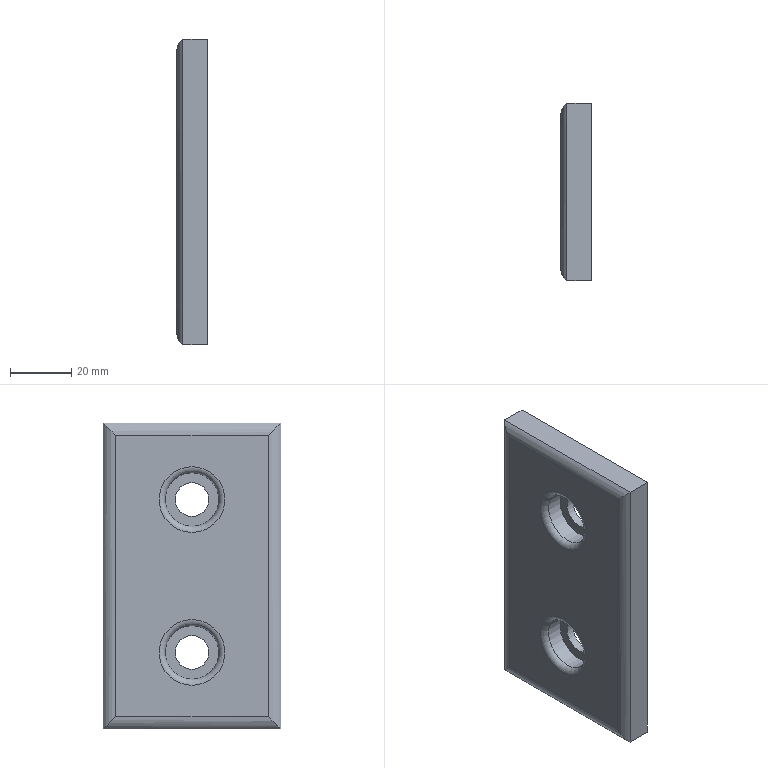Part | STEP file | lll_id5046_x_t | 1 solid | 18 faces | box 10 x 58 x 100 mm | volume 53133 mm3 | plane 8 | cylinder 8 | torus 2 | commonest cylinder face diameters 10 x4 11 x2 17.5 x2
STEP:
#1=CARTESIAN_POINT('',(2835.,334.047,9.));
#2=VERTEX_POINT('',#1);
#3=CARTESIAN_POINT('',(2835.,284.047,9.));
#4=VERTEX_POINT('',#3);
#5=CARTESIAN_POINT('',(2835.,323.047,9.));
#6=DIRECTION('',(0.,-1.,0.));
#7=VECTOR('',#6,1.);
#8=LINE('',#5,#7);
#9=EDGE_CURVE('',#2,#4,#8,.T.);
#10=ORIENTED_EDGE('',*,*,#9,.T.);
#11=CARTESIAN_POINT('',(2835.,284.047,101.));
#12=VERTEX_POINT('',#11);
#13=CARTESIAN_POINT('',(2835.,284.047,105.));
#14=DIRECTION('',(0.,0.,-1.));
#15=VECTOR('',#14,1.);
#16=LINE('',#13,#15);
#17=EDGE_CURVE('',#12,#4,#16,.T.);
#18=ORIENTED_EDGE('',*,*,#17,.F.);
#19=CARTESIAN_POINT('',(2835.,334.047,101.));
#20=VERTEX_POINT('',#19);
#21=CARTESIAN_POINT('',(2835.,323.047,101.));
#22=DIRECTION('',(0.,-1.,0.));
#23=VECTOR('',#22,1.);
#24=LINE('',#21,#23);
#25=EDGE_CURVE('',#20,#12,#24,.T.);
#26=ORIENTED_EDGE('',*,*,#25,.F.);
#27=CARTESIAN_POINT('',(2835.,334.047,105.));
#28=DIRECTION('',(0.,0.,-1.));
#29=VECTOR('',#28,1.);
#30=LINE('',#27,#29);
#31=EDGE_CURVE('',#20,#2,#30,.T.);
#32=ORIENTED_EDGE('',*,*,#31,.T.);
#33=EDGE_LOOP('',(#10,#18,#26,#32));
#34=FACE_BOUND('',#33,.T.);
#35=CARTESIAN_POINT('',(2835.,309.047,69.25));
#36=VERTEX_POINT('',#35);
#37=CARTESIAN_POINT('',(2835.,309.047,80.));
#38=DIRECTION('',(1.,0.,0.));
#39=DIRECTION('',(0.,0.,-1.));
#40=AXIS2_PLACEMENT_3D('',#37,#38,#39);
#41=CIRCLE('',#40,10.75);
#42=EDGE_CURVE('',#36,#36,#41,.T.);
#43=ORIENTED_EDGE('',*,*,#42,.T.);
#44=EDGE_LOOP('',(#43));
#45=FACE_BOUND('',#44,.T.);
#46=CARTESIAN_POINT('',(2835.,309.047,19.25));
#47=VERTEX_POINT('',#46);
#48=CARTESIAN_POINT('',(2835.,309.047,30.));
#49=DIRECTION('',(1.,0.,0.));
#50=DIRECTION('',(0.,0.,-1.));
#51=AXIS2_PLACEMENT_3D('',#48,#49,#50);
#52=CIRCLE('',#51,10.75);
#53=EDGE_CURVE('',#47,#47,#52,.T.);
#54=ORIENTED_EDGE('',*,*,#53,.T.);
#55=EDGE_LOOP('',(#54));
#56=FACE_BOUND('',#55,.T.);
#57=CARTESIAN_POINT('',(2835.,295.047,-20.));
#58=DIRECTION('',(-1.,0.,0.));
#59=DIRECTION('',(0.,0.,-1.));
#60=AXIS2_PLACEMENT_3D('',#57,#58,#59);
#61=PLANE('',#60);
#62=ADVANCED_FACE('',(#34,#45,#56),#61,.T.);
#63=CARTESIAN_POINT('',(2845.,309.047,24.5));
#64=VERTEX_POINT('',#63);
#65=CARTESIAN_POINT('',(2845.,309.047,30.));
#66=DIRECTION('',(1.,0.,0.));
#67=DIRECTION('',(0.,0.,-1.));
#68=AXIS2_PLACEMENT_3D('',#65,#66,#67);
#69=CIRCLE('',#68,5.5);
#70=EDGE_CURVE('',#64,#64,#69,.T.);
#71=ORIENTED_EDGE('',*,*,#70,.T.);
#72=EDGE_LOOP('',(#71));
#73=FACE_BOUND('',#72,.T.);
#74=CARTESIAN_POINT('',(2842.3,309.047,24.5));
#75=VERTEX_POINT('',#74);
#76=CARTESIAN_POINT('',(2842.3,309.047,30.));
#77=DIRECTION('',(1.,0.,0.));
#78=DIRECTION('',(0.,0.,-1.));
#79=AXIS2_PLACEMENT_3D('',#76,#77,#78);
#80=CIRCLE('',#79,5.5);
#81=EDGE_CURVE('',#75,#75,#80,.T.);
#82=ORIENTED_EDGE('',*,*,#81,.F.);
#83=EDGE_LOOP('',(#82));
#84=FACE_BOUND('',#83,.T.);
#85=CARTESIAN_POINT('',(2934.,309.047,30.));
#86=DIRECTION('',(-1.,0.,0.));
#87=DIRECTION('',(0.,0.,-1.));
#88=AXIS2_PLACEMENT_3D('',#85,#86,#87);
#89=CYLINDRICAL_SURFACE('',#88,5.5);
#90=ADVANCED_FACE('',(#73,#84),#89,.F.);
#91=CARTESIAN_POINT('',(2845.,338.047,5.));
#92=VERTEX_POINT('',#91);
#93=CARTESIAN_POINT('',(2845.,280.047,5.));
#94=VERTEX_POINT('',#93);
#95=CARTESIAN_POINT('',(2845.,323.047,5.));
#96=DIRECTION('',(0.,-1.,0.));
#97=VECTOR('',#96,1.);
#98=LINE('',#95,#97);
#99=EDGE_CURVE('',#92,#94,#98,.T.);
#100=ORIENTED_EDGE('',*,*,#99,.F.);
#101=CARTESIAN_POINT('',(2845.,338.047,105.));
#102=VERTEX_POINT('',#101);
#103=CARTESIAN_POINT('',(2845.,338.047,105.));
#104=DIRECTION('',(0.,0.,-1.));
#105=VECTOR('',#104,1.);
#106=LINE('',#103,#105);
#107=EDGE_CURVE('',#102,#92,#106,.T.);
#108=ORIENTED_EDGE('',*,*,#107,.F.);
#109=CARTESIAN_POINT('',(2845.,280.047,105.));
#110=VERTEX_POINT('',#109);
#111=CARTESIAN_POINT('',(2845.,295.047,105.));
#112=DIRECTION('',(0.,1.,0.));
#113=VECTOR('',#112,1.);
#114=LINE('',#111,#113);
#115=EDGE_CURVE('',#110,#102,#114,.T.);
#116=ORIENTED_EDGE('',*,*,#115,.F.);
#117=CARTESIAN_POINT('',(2845.,280.047,-20.));
#118=DIRECTION('',(0.,0.,1.));
#119=VECTOR('',#118,1.);
#120=LINE('',#117,#119);
#121=EDGE_CURVE('',#94,#110,#120,.T.);
#122=ORIENTED_EDGE('',*,*,#121,.F.);
#123=EDGE_LOOP('',(#100,#108,#116,#122));
#124=FACE_BOUND('',#123,.T.);
#125=ORIENTED_EDGE('',*,*,#70,.F.);
#126=EDGE_LOOP('',(#125));
#127=FACE_BOUND('',#126,.T.);
#128=CARTESIAN_POINT('',(2845.,309.047,74.5));
#129=VERTEX_POINT('',#128);
#130=CARTESIAN_POINT('',(2845.,309.047,80.));
#131=DIRECTION('',(-1.,0.,0.));
#132=DIRECTION('',(0.,0.,-1.));
#133=AXIS2_PLACEMENT_3D('',#130,#131,#132);
#134=CIRCLE('',#133,5.5);
#135=EDGE_CURVE('',#129,#129,#134,.T.);
#136=ORIENTED_EDGE('',*,*,#135,.T.);
#137=EDGE_LOOP('',(#136));
#138=FACE_BOUND('',#137,.T.);
#139=CARTESIAN_POINT('',(2845.,295.047,-20.));
#140=DIRECTION('',(-1.,0.,0.));
#141=DIRECTION('',(0.,0.,-1.));
#142=AXIS2_PLACEMENT_3D('',#139,#140,#141);
#143=PLANE('',#142);
#144=ADVANCED_FACE('',(#124,#127,#138),#143,.F.);
#145=CARTESIAN_POINT('',(2837.,280.047,105.));
#146=VERTEX_POINT('',#145);
#147=CARTESIAN_POINT('',(2835.,280.047,105.));
#148=DIRECTION('',(1.,0.,0.));
#149=VECTOR('',#148,1.);
#150=LINE('',#147,#149);
#151=EDGE_CURVE('',#146,#110,#150,.T.);
#152=ORIENTED_EDGE('',*,*,#151,.F.);
#153=CARTESIAN_POINT('',(2837.,280.047,5.));
#154=VERTEX_POINT('',#153);
#155=CARTESIAN_POINT('',(2837.,280.047,105.));
#156=DIRECTION('',(0.,0.,-1.));
#157=VECTOR('',#156,1.);
#158=LINE('',#155,#157);
#159=EDGE_CURVE('',#146,#154,#158,.T.);
#160=ORIENTED_EDGE('',*,*,#159,.T.);
#161=CARTESIAN_POINT('',(2835.,280.047,5.));
#162=DIRECTION('',(1.,0.,0.));
#163=VECTOR('',#162,1.);
#164=LINE('',#161,#163);
#165=EDGE_CURVE('',#154,#94,#164,.T.);
#166=ORIENTED_EDGE('',*,*,#165,.T.);
#167=ORIENTED_EDGE('',*,*,#121,.T.);
#168=EDGE_LOOP('',(#152,#160,#166,#167));
#169=FACE_OUTER_BOUND('',#168,.T.);
#170=CARTESIAN_POINT('',(2835.,280.047,-20.));
#171=DIRECTION('',(0.,1.,0.));
#172=DIRECTION('',(1.,0.,0.));
#173=AXIS2_PLACEMENT_3D('',#170,#171,#172);
#174=PLANE('',#173);
#175=ADVANCED_FACE('',(#169),#174,.F.);
#176=CARTESIAN_POINT('',(2837.,338.047,105.));
#177=VERTEX_POINT('',#176);
#178=CARTESIAN_POINT('',(2837.,323.047,105.));
#179=DIRECTION('',(0.,-1.,0.));
#180=VECTOR('',#179,1.);
#181=LINE('',#178,#180);
#182=EDGE_CURVE('',#177,#146,#181,.T.);
#183=ORIENTED_EDGE('',*,*,#182,.T.);
#184=ORIENTED_EDGE('',*,*,#151,.T.);
#185=ORIENTED_EDGE('',*,*,#115,.T.);
#186=CARTESIAN_POINT('',(2835.,338.047,105.));
#187=DIRECTION('',(1.,0.,0.));
#188=VECTOR('',#187,1.);
#189=LINE('',#186,#188);
#190=EDGE_CURVE('',#177,#102,#189,.T.);
#191=ORIENTED_EDGE('',*,*,#190,.F.);
#192=EDGE_LOOP('',(#183,#184,#185,#191));
#193=FACE_OUTER_BOUND('',#192,.T.);
#194=CARTESIAN_POINT('',(2835.,295.047,105.));
#195=DIRECTION('',(0.,0.,-1.));
#196=DIRECTION('',(1.,0.,0.));
#197=AXIS2_PLACEMENT_3D('',#194,#195,#196);
#198=PLANE('',#197);
#199=ADVANCED_FACE('',(#193),#198,.F.);
#200=CARTESIAN_POINT('',(2837.,338.047,5.));
#201=VERTEX_POINT('',#200);
#202=CARTESIAN_POINT('',(2835.,338.047,5.));
#203=DIRECTION('',(1.,0.,0.));
#204=VECTOR('',#203,1.);
#205=LINE('',#202,#204);
#206=EDGE_CURVE('',#201,#92,#205,.T.);
#207=ORIENTED_EDGE('',*,*,#206,.F.);
#208=CARTESIAN_POINT('',(2837.,338.047,105.));
#209=DIRECTION('',(0.,0.,-1.));
#210=VECTOR('',#209,1.);
#211=LINE('',#208,#210);
#212=EDGE_CURVE('',#177,#201,#211,.T.);
#213=ORIENTED_EDGE('',*,*,#212,.F.);
#214=ORIENTED_EDGE('',*,*,#190,.T.);
#215=ORIENTED_EDGE('',*,*,#107,.T.);
#216=EDGE_LOOP('',(#207,#213,#214,#215));
#217=FACE_OUTER_BOUND('',#216,.T.);
#218=CARTESIAN_POINT('',(2835.,338.047,105.));
#219=DIRECTION('',(0.,-1.,0.));
#220=DIRECTION('',(-1.,0.,0.));
#221=AXIS2_PLACEMENT_3D('',#218,#219,#220);
#222=PLANE('',#221);
#223=ADVANCED_FACE('',(#217),#222,.F.);
#224=ORIENTED_EDGE('',*,*,#165,.F.);
#225=CARTESIAN_POINT('',(2837.,323.047,5.));
#226=DIRECTION('',(0.,-1.,0.));
#227=VECTOR('',#226,1.);
#228=LINE('',#225,#227);
#229=EDGE_CURVE('',#201,#154,#228,.T.);
#230=ORIENTED_EDGE('',*,*,#229,.F.);
#231=ORIENTED_EDGE('',*,*,#206,.T.);
#232=ORIENTED_EDGE('',*,*,#99,.T.);
#233=EDGE_LOOP('',(#224,#230,#231,#232));
#234=FACE_OUTER_BOUND('',#233,.T.);
#235=CARTESIAN_POINT('',(2835.,323.047,5.));
#236=DIRECTION('',(0.,0.,1.));
#237=DIRECTION('',(-1.,0.,0.));
#238=AXIS2_PLACEMENT_3D('',#235,#236,#237);
#239=PLANE('',#238);
#240=ADVANCED_FACE('',(#234),#239,.F.);
#241=CARTESIAN_POINT('',(2840.,334.047,101.));
#242=DIRECTION('',(0.,0.7071,-0.7071));
#243=DIRECTION('',(0.,-0.7071,-0.7071));
#244=AXIS2_PLACEMENT_3D('',#241,#242,#243);
#245=ELLIPSE('',#244,7.071,5.);
#246=EDGE_CURVE('',#20,#177,#245,.T.);
#247=ORIENTED_EDGE('',*,*,#246,.F.);
#248=ORIENTED_EDGE('',*,*,#25,.T.);
#249=CARTESIAN_POINT('',(2840.,284.047,101.));
#250=DIRECTION('',(0.,-0.7071,-0.7071));
#251=DIRECTION('',(0.,-0.7071,0.7071));
#252=AXIS2_PLACEMENT_3D('',#249,#250,#251);
#253=ELLIPSE('',#252,7.071,5.);
#254=EDGE_CURVE('',#146,#12,#253,.T.);
#255=ORIENTED_EDGE('',*,*,#254,.F.);
#256=ORIENTED_EDGE('',*,*,#182,.F.);
#257=EDGE_LOOP('',(#247,#248,#255,#256));
#258=FACE_OUTER_BOUND('',#257,.T.);
#259=CARTESIAN_POINT('',(2840.,323.047,101.));
#260=DIRECTION('',(0.,-1.,0.));
#261=DIRECTION('',(-1.,0.,0.));
#262=AXIS2_PLACEMENT_3D('',#259,#260,#261);
#263=CYLINDRICAL_SURFACE('',#262,5.);
#264=ADVANCED_FACE('',(#258),#263,.T.);
#265=ORIENTED_EDGE('',*,*,#17,.T.);
#266=CARTESIAN_POINT('',(2840.,284.047,9.));
#267=DIRECTION('',(0.,-0.7071,0.7071));
#268=DIRECTION('',(0.,-0.7071,-0.7071));
#269=AXIS2_PLACEMENT_3D('',#266,#267,#268);
#270=ELLIPSE('',#269,7.071,5.);
#271=EDGE_CURVE('',#4,#154,#270,.T.);
#272=ORIENTED_EDGE('',*,*,#271,.T.);
#273=ORIENTED_EDGE('',*,*,#159,.F.);
#274=ORIENTED_EDGE('',*,*,#254,.T.);
#275=EDGE_LOOP('',(#265,#272,#273,#274));
#276=FACE_OUTER_BOUND('',#275,.T.);
#277=CARTESIAN_POINT('',(2840.,284.047,105.));
#278=DIRECTION('',(0.,0.,-1.));
#279=DIRECTION('',(1.,0.,0.));
#280=AXIS2_PLACEMENT_3D('',#277,#278,#279);
#281=CYLINDRICAL_SURFACE('',#280,5.);
#282=ADVANCED_FACE('',(#276),#281,.T.);
#283=CARTESIAN_POINT('',(2840.,334.047,9.));
#284=DIRECTION('',(0.,0.7071,0.7071));
#285=DIRECTION('',(0.,0.7071,-0.7071));
#286=AXIS2_PLACEMENT_3D('',#283,#284,#285);
#287=ELLIPSE('',#286,7.071,5.);
#288=EDGE_CURVE('',#201,#2,#287,.T.);
#289=ORIENTED_EDGE('',*,*,#288,.T.);
#290=ORIENTED_EDGE('',*,*,#31,.F.);
#291=ORIENTED_EDGE('',*,*,#246,.T.);
#292=ORIENTED_EDGE('',*,*,#212,.T.);
#293=EDGE_LOOP('',(#289,#290,#291,#292));
#294=FACE_OUTER_BOUND('',#293,.T.);
#295=CARTESIAN_POINT('',(2840.,334.047,105.));
#296=DIRECTION('',(0.,0.,-1.));
#297=DIRECTION('',(1.,0.,0.));
#298=AXIS2_PLACEMENT_3D('',#295,#296,#297);
#299=CYLINDRICAL_SURFACE('',#298,5.);
#300=ADVANCED_FACE('',(#294),#299,.T.);
#301=ORIENTED_EDGE('',*,*,#271,.F.);
#302=ORIENTED_EDGE('',*,*,#9,.F.);
#303=ORIENTED_EDGE('',*,*,#288,.F.);
#304=ORIENTED_EDGE('',*,*,#229,.T.);
#305=EDGE_LOOP('',(#301,#302,#303,#304));
#306=FACE_OUTER_BOUND('',#305,.T.);
#307=CARTESIAN_POINT('',(2840.,323.047,9.));
#308=DIRECTION('',(0.,-1.,0.));
#309=DIRECTION('',(-1.,0.,0.));
#310=AXIS2_PLACEMENT_3D('',#307,#308,#309);
#311=CYLINDRICAL_SURFACE('',#310,5.);
#312=ADVANCED_FACE('',(#306),#311,.T.);
#313=CARTESIAN_POINT('',(2842.3,309.047,85.5));
#314=VERTEX_POINT('',#313);
#315=CARTESIAN_POINT('',(2842.3,309.047,80.));
#316=DIRECTION('',(1.,0.,0.));
#317=DIRECTION('',(0.,0.,1.));
#318=AXIS2_PLACEMENT_3D('',#315,#316,#317);
#319=CIRCLE('',#318,5.5);
#320=EDGE_CURVE('',#314,#314,#319,.T.);
#321=ORIENTED_EDGE('',*,*,#320,.F.);
#322=EDGE_LOOP('',(#321));
#323=FACE_BOUND('',#322,.T.);
#324=ORIENTED_EDGE('',*,*,#135,.F.);
#325=EDGE_LOOP('',(#324));
#326=FACE_BOUND('',#325,.T.);
#327=CARTESIAN_POINT('',(2934.,309.047,80.));
#328=DIRECTION('',(-1.,0.,0.));
#329=DIRECTION('',(0.,0.,-1.));
#330=AXIS2_PLACEMENT_3D('',#327,#328,#329);
#331=CYLINDRICAL_SURFACE('',#330,5.5);
#332=ADVANCED_FACE('',(#323,#326),#331,.F.);
#333=CARTESIAN_POINT('',(2842.3,309.047,21.25));
#334=VERTEX_POINT('',#333);
#335=CARTESIAN_POINT('',(2842.3,309.047,30.));
#336=DIRECTION('',(1.,0.,0.));
#337=DIRECTION('',(0.,0.,-1.));
#338=AXIS2_PLACEMENT_3D('',#335,#336,#337);
#339=CIRCLE('',#338,8.75);
#340=EDGE_CURVE('',#334,#334,#339,.T.);
#341=ORIENTED_EDGE('',*,*,#340,.F.);
#342=EDGE_LOOP('',(#341));
#343=FACE_BOUND('',#342,.T.);
#344=ORIENTED_EDGE('',*,*,#81,.T.);
#345=EDGE_LOOP('',(#344));
#346=FACE_BOUND('',#345,.T.);
#347=CARTESIAN_POINT('',(2842.3,309.047,30.));
#348=DIRECTION('',(-1.,0.,0.));
#349=DIRECTION('',(0.,0.,-1.));
#350=AXIS2_PLACEMENT_3D('',#347,#348,#349);
#351=PLANE('',#350);
#352=ADVANCED_FACE('',(#343,#346),#351,.T.);
#353=CARTESIAN_POINT('',(2837.,309.047,21.25));
#354=VERTEX_POINT('',#353);
#355=CARTESIAN_POINT('',(2837.,309.047,30.));
#356=DIRECTION('',(-1.,0.,0.));
#357=DIRECTION('',(0.,0.,-1.));
#358=AXIS2_PLACEMENT_3D('',#355,#356,#357);
#359=CIRCLE('',#358,8.75);
#360=EDGE_CURVE('',#354,#354,#359,.T.);
#361=ORIENTED_EDGE('',*,*,#360,.T.);
#362=EDGE_LOOP('',(#361));
#363=FACE_BOUND('',#362,.T.);
#364=ORIENTED_EDGE('',*,*,#340,.T.);
#365=EDGE_LOOP('',(#364));
#366=FACE_BOUND('',#365,.T.);
#367=CARTESIAN_POINT('',(2842.3,309.047,30.));
#368=DIRECTION('',(-1.,0.,0.));
#369=DIRECTION('',(0.,0.,-1.));
#370=AXIS2_PLACEMENT_3D('',#367,#368,#369);
#371=CYLINDRICAL_SURFACE('',#370,8.75);
#372=ADVANCED_FACE('',(#363,#366),#371,.F.);
#373=CARTESIAN_POINT('',(2837.,309.047,71.25));
#374=VERTEX_POINT('',#373);
#375=CARTESIAN_POINT('',(2837.,309.047,80.));
#376=DIRECTION('',(-1.,0.,0.));
#377=DIRECTION('',(0.,0.,-1.));
#378=AXIS2_PLACEMENT_3D('',#375,#376,#377);
#379=CIRCLE('',#378,8.75);
#380=EDGE_CURVE('',#374,#374,#379,.T.);
#381=ORIENTED_EDGE('',*,*,#380,.T.);
#382=EDGE_LOOP('',(#381));
#383=FACE_BOUND('',#382,.T.);
#384=CARTESIAN_POINT('',(2842.3,309.047,71.25));
#385=VERTEX_POINT('',#384);
#386=CARTESIAN_POINT('',(2842.3,309.047,80.));
#387=DIRECTION('',(-1.,0.,0.));
#388=DIRECTION('',(0.,0.,-1.));
#389=AXIS2_PLACEMENT_3D('',#386,#387,#388);
#390=CIRCLE('',#389,8.75);
#391=EDGE_CURVE('',#385,#385,#390,.T.);
#392=ORIENTED_EDGE('',*,*,#391,.F.);
#393=EDGE_LOOP('',(#392));
#394=FACE_BOUND('',#393,.T.);
#395=CARTESIAN_POINT('',(2842.3,309.047,80.));
#396=DIRECTION('',(-1.,0.,0.));
#397=DIRECTION('',(0.,0.,-1.));
#398=AXIS2_PLACEMENT_3D('',#395,#396,#397);
#399=CYLINDRICAL_SURFACE('',#398,8.75);
#400=ADVANCED_FACE('',(#383,#394),#399,.F.);
#401=ORIENTED_EDGE('',*,*,#320,.T.);
#402=EDGE_LOOP('',(#401));
#403=FACE_BOUND('',#402,.T.);
#404=ORIENTED_EDGE('',*,*,#391,.T.);
#405=EDGE_LOOP('',(#404));
#406=FACE_BOUND('',#405,.T.);
#407=CARTESIAN_POINT('',(2842.3,309.047,80.));
#408=DIRECTION('',(1.,0.,0.));
#409=DIRECTION('',(0.,0.,1.));
#410=AXIS2_PLACEMENT_3D('',#407,#408,#409);
#411=PLANE('',#410);
#412=ADVANCED_FACE('',(#403,#406),#411,.F.);
#413=ORIENTED_EDGE('',*,*,#53,.F.);
#414=EDGE_LOOP('',(#413));
#415=FACE_BOUND('',#414,.T.);
#416=ORIENTED_EDGE('',*,*,#360,.F.);
#417=EDGE_LOOP('',(#416));
#418=FACE_BOUND('',#417,.T.);
#419=CARTESIAN_POINT('',(2837.,309.047,30.));
#420=DIRECTION('',(-1.,0.,0.));
#421=DIRECTION('',(0.,0.,-1.));
#422=AXIS2_PLACEMENT_3D('',#419,#420,#421);
#423=TOROIDAL_SURFACE('',#422,10.75,2.);
#424=ADVANCED_FACE('',(#415,#418),#423,.T.);
#425=ORIENTED_EDGE('',*,*,#380,.F.);
#426=EDGE_LOOP('',(#425));
#427=FACE_BOUND('',#426,.T.);
#428=ORIENTED_EDGE('',*,*,#42,.F.);
#429=EDGE_LOOP('',(#428));
#430=FACE_BOUND('',#429,.T.);
#431=CARTESIAN_POINT('',(2837.,309.047,80.));
#432=DIRECTION('',(-1.,0.,0.));
#433=DIRECTION('',(0.,0.,-1.));
#434=AXIS2_PLACEMENT_3D('',#431,#432,#433);
#435=TOROIDAL_SURFACE('',#434,10.75,2.);
#436=ADVANCED_FACE('',(#427,#430),#435,.T.);
#437=CLOSED_SHELL('',(#62,#90,#144,#175,#199,#223,#240,#264,#282,#300,#312,#332,#352,#372,#400,#412,#424,#436));
#438=MANIFOLD_SOLID_BREP('',#437);
#439=(LENGTH_UNIT()NAMED_UNIT(*)SI_UNIT(.MILLI.,.METRE.));
#440=UNCERTAINTY_MEASURE_WITH_UNIT(LENGTH_MEASURE(0.00002),#439,'','');
#441=(NAMED_UNIT(*)PLANE_ANGLE_UNIT()SI_UNIT($,.RADIAN.));
#442=PLANE_ANGLE_MEASURE_WITH_UNIT(PLANE_ANGLE_MEASURE(0.01745),#441);
#443=DIMENSIONAL_EXPONENTS(0.,0.,0.,0.,0.,0.,0.);
#444=(CONVERSION_BASED_UNIT('DEGREE',#442)NAMED_UNIT(#443)PLANE_ANGLE_UNIT());
#445=(NAMED_UNIT(*)SI_UNIT($,.STERADIAN.)SOLID_ANGLE_UNIT());
#446=(GEOMETRIC_REPRESENTATION_CONTEXT(3)GLOBAL_UNCERTAINTY_ASSIGNED_CONTEXT((#440))GLOBAL_UNIT_ASSIGNED_CONTEXT((#439,#444,#445))REPRESENTATION_CONTEXT('',''));
#447=ADVANCED_BREP_SHAPE_REPRESENTATION('',(#438),#446);